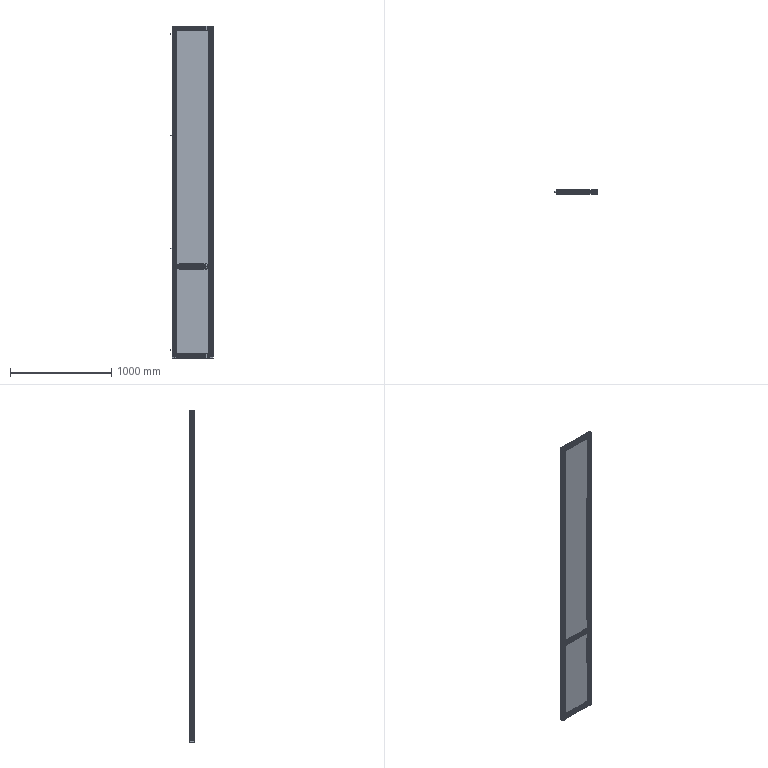Part | SolidWorks | features ReferencePattern 12, LocalLPattern 4 | 67 solids | 3410 faces | volume 10335733 mm3 | plane 2303 | cylinder 935 | cone 140 | spline 32 | commonest cylinder face diameters 0.562 x120 5 x104 6.8 x103 11 x56 2 x54 8 x48